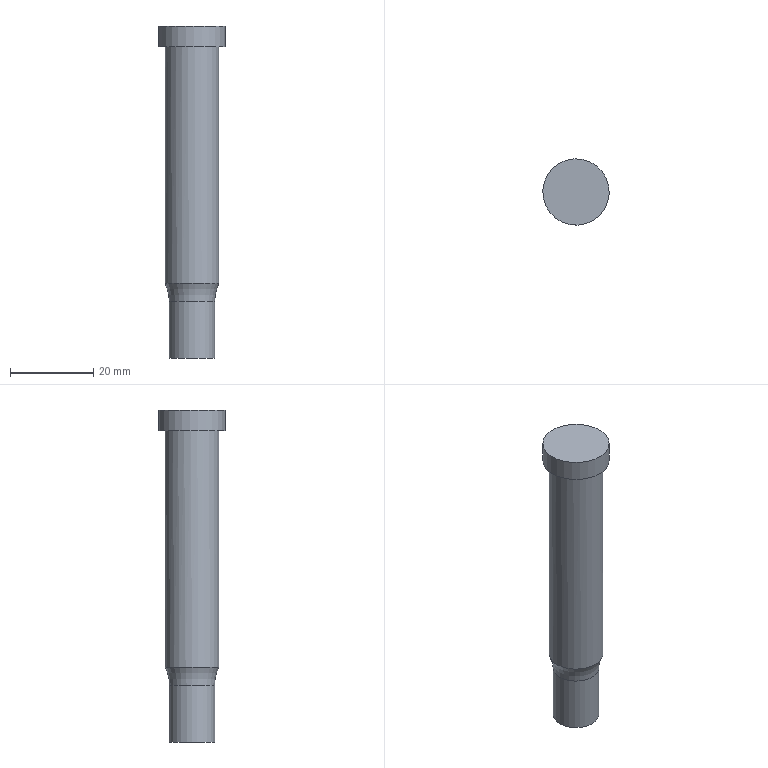Part | NX | features MAIN_BODY 2 | 1 solid | 7 faces | box 16 x 16 x 80 mm | volume 10333 mm3 | cylinder 3 | plane 3 | torus 1 | commonest cylinder face diameters 11 x1 13 x1 16 x1
STEP:
#1=CARTESIAN_POINT('',(1593.5,26.952,39.975));
#2=VERTEX_POINT('',#1);
#3=CARTESIAN_POINT('',(1587.,26.952,39.975));
#4=DIRECTION('',(0.,0.,1.));
#5=DIRECTION('',(1.,0.,0.));
#6=AXIS2_PLACEMENT_3D('',#3,#4,#5);
#7=CIRCLE('',#6,6.5);
#8=EDGE_CURVE('',#2,#2,#7,.F.);
#9=ORIENTED_EDGE('',*,*,#8,.F.);
#10=EDGE_LOOP('',(#9));
#11=FACE_BOUND('',#10,.T.);
#12=CARTESIAN_POINT('',(1582.404,31.549,97.));
#13=VERTEX_POINT('',#12);
#14=CARTESIAN_POINT('',(1587.,26.952,97.));
#15=DIRECTION('',(0.,0.,-1.));
#16=DIRECTION('',(-0.7071,0.7071,0.));
#17=AXIS2_PLACEMENT_3D('',#14,#15,#16);
#18=CIRCLE('',#17,6.5);
#19=EDGE_CURVE('',#13,#13,#18,.T.);
#20=ORIENTED_EDGE('',*,*,#19,.T.);
#21=EDGE_LOOP('',(#20));
#22=FACE_BOUND('',#21,.T.);
#23=CARTESIAN_POINT('',(1587.,26.952,102.));
#24=DIRECTION('',(0.,0.,-1.));
#25=DIRECTION('',(0.7071,-0.7071,0.));
#26=AXIS2_PLACEMENT_3D('',#23,#24,#25);
#27=CYLINDRICAL_SURFACE('',#26,6.5);
#28=ADVANCED_FACE('',(#11,#22),#27,.T.);
#29=CARTESIAN_POINT('',(1581.343,32.609,97.));
#30=VERTEX_POINT('',#29);
#31=CARTESIAN_POINT('',(1587.,26.952,97.));
#32=DIRECTION('',(0.,0.,-1.));
#33=DIRECTION('',(-0.7071,0.7071,0.));
#34=AXIS2_PLACEMENT_3D('',#31,#32,#33);
#35=CIRCLE('',#34,8.);
#36=EDGE_CURVE('',#30,#30,#35,.T.);
#37=ORIENTED_EDGE('',*,*,#36,.T.);
#38=EDGE_LOOP('',(#37));
#39=FACE_BOUND('',#38,.T.);
#40=ORIENTED_EDGE('',*,*,#19,.F.);
#41=EDGE_LOOP('',(#40));
#42=FACE_BOUND('',#41,.T.);
#43=CARTESIAN_POINT('',(1587.,26.952,97.));
#44=DIRECTION('',(0.,0.,1.));
#45=DIRECTION('',(-0.7071,0.7071,0.));
#46=AXIS2_PLACEMENT_3D('',#43,#44,#45);
#47=PLANE('',#46);
#48=ADVANCED_FACE('',(#39,#42),#47,.F.);
#49=ORIENTED_EDGE('',*,*,#36,.F.);
#50=EDGE_LOOP('',(#49));
#51=FACE_BOUND('',#50,.T.);
#52=CARTESIAN_POINT('',(1581.343,32.609,102.));
#53=VERTEX_POINT('',#52);
#54=CARTESIAN_POINT('',(1587.,26.952,102.));
#55=DIRECTION('',(0.,0.,-1.));
#56=DIRECTION('',(-0.7071,0.7071,0.));
#57=AXIS2_PLACEMENT_3D('',#54,#55,#56);
#58=CIRCLE('',#57,8.);
#59=EDGE_CURVE('',#53,#53,#58,.T.);
#60=ORIENTED_EDGE('',*,*,#59,.T.);
#61=EDGE_LOOP('',(#60));
#62=FACE_BOUND('',#61,.T.);
#63=CARTESIAN_POINT('',(1587.,26.952,98.));
#64=DIRECTION('',(0.,0.,1.));
#65=DIRECTION('',(-0.7071,0.7071,0.));
#66=AXIS2_PLACEMENT_3D('',#63,#64,#65);
#67=CYLINDRICAL_SURFACE('',#66,8.);
#68=ADVANCED_FACE('',(#51,#62),#67,.T.);
#69=ORIENTED_EDGE('',*,*,#59,.F.);
#70=EDGE_LOOP('',(#69));
#71=FACE_BOUND('',#70,.T.);
#72=CARTESIAN_POINT('',(1587.,26.952,102.));
#73=DIRECTION('',(0.,0.,1.));
#74=DIRECTION('',(-0.7071,0.7071,0.));
#75=AXIS2_PLACEMENT_3D('',#72,#73,#74);
#76=PLANE('',#75);
#77=ADVANCED_FACE('',(#71),#76,.T.);
#78=CARTESIAN_POINT('',(1581.5,26.952,35.732));
#79=VERTEX_POINT('',#78);
#80=CARTESIAN_POINT('',(1587.,26.952,35.732));
#81=DIRECTION('',(0.,0.,-1.));
#82=DIRECTION('',(-1.,0.,0.));
#83=AXIS2_PLACEMENT_3D('',#80,#81,#82);
#84=CIRCLE('',#83,5.5);
#85=EDGE_CURVE('',#79,#79,#84,.F.);
#86=ORIENTED_EDGE('',*,*,#85,.F.);
#87=EDGE_LOOP('',(#86));
#88=FACE_BOUND('',#87,.T.);
#89=CARTESIAN_POINT('',(1581.5,26.952,22.));
#90=VERTEX_POINT('',#89);
#91=CARTESIAN_POINT('',(1587.,26.952,22.));
#92=DIRECTION('',(0.,0.,-1.));
#93=DIRECTION('',(-1.,0.,0.));
#94=AXIS2_PLACEMENT_3D('',#91,#92,#93);
#95=CIRCLE('',#94,5.5);
#96=EDGE_CURVE('',#90,#90,#95,.T.);
#97=ORIENTED_EDGE('',*,*,#96,.F.);
#98=EDGE_LOOP('',(#97));
#99=FACE_BOUND('',#98,.T.);
#100=CARTESIAN_POINT('',(1587.,26.952,22.));
#101=DIRECTION('',(0.,0.,1.));
#102=DIRECTION('',(-0.7071,0.7071,0.));
#103=AXIS2_PLACEMENT_3D('',#100,#101,#102);
#104=CYLINDRICAL_SURFACE('',#103,5.5);
#105=ADVANCED_FACE('',(#88,#99),#104,.T.);
#106=ORIENTED_EDGE('',*,*,#96,.T.);
#107=EDGE_LOOP('',(#106));
#108=FACE_BOUND('',#107,.T.);
#109=CARTESIAN_POINT('',(1587.,26.952,22.));
#110=DIRECTION('',(0.,0.,1.));
#111=DIRECTION('',(-0.7071,0.7071,0.));
#112=AXIS2_PLACEMENT_3D('',#109,#110,#111);
#113=PLANE('',#112);
#114=ADVANCED_FACE('',(#108),#113,.F.);
#115=ORIENTED_EDGE('',*,*,#85,.T.);
#116=EDGE_LOOP('',(#115));
#117=FACE_BOUND('',#116,.T.);
#118=ORIENTED_EDGE('',*,*,#8,.T.);
#119=EDGE_LOOP('',(#118));
#120=FACE_BOUND('',#119,.T.);
#121=CARTESIAN_POINT('',(1587.,26.952,35.732));
#122=DIRECTION('',(0.,0.,1.));
#123=DIRECTION('',(-0.7071,0.7071,0.));
#124=AXIS2_PLACEMENT_3D('',#121,#122,#123);
#125=TOROIDAL_SURFACE('',#124,15.,9.5);
#126=ADVANCED_FACE('',(#117,#120),#125,.F.);
#127=CLOSED_SHELL('',(#28,#48,#68,#77,#105,#114,#126));
#128=MANIFOLD_SOLID_BREP('',#127);
#129=(LENGTH_UNIT()NAMED_UNIT(*)SI_UNIT(.MILLI.,.METRE.));
#130=UNCERTAINTY_MEASURE_WITH_UNIT(LENGTH_MEASURE(0.00001),#129,'','');
#131=(NAMED_UNIT(*)PLANE_ANGLE_UNIT()SI_UNIT($,.RADIAN.));
#132=(NAMED_UNIT(*)SI_UNIT($,.STERADIAN.)SOLID_ANGLE_UNIT());
#133=(GEOMETRIC_REPRESENTATION_CONTEXT(3)GLOBAL_UNCERTAINTY_ASSIGNED_CONTEXT((#130))GLOBAL_UNIT_ASSIGNED_CONTEXT((#129,#131,#132))REPRESENTATION_CONTEXT('',''));
#134=ADVANCED_BREP_SHAPE_REPRESENTATION('',(#128),#133);